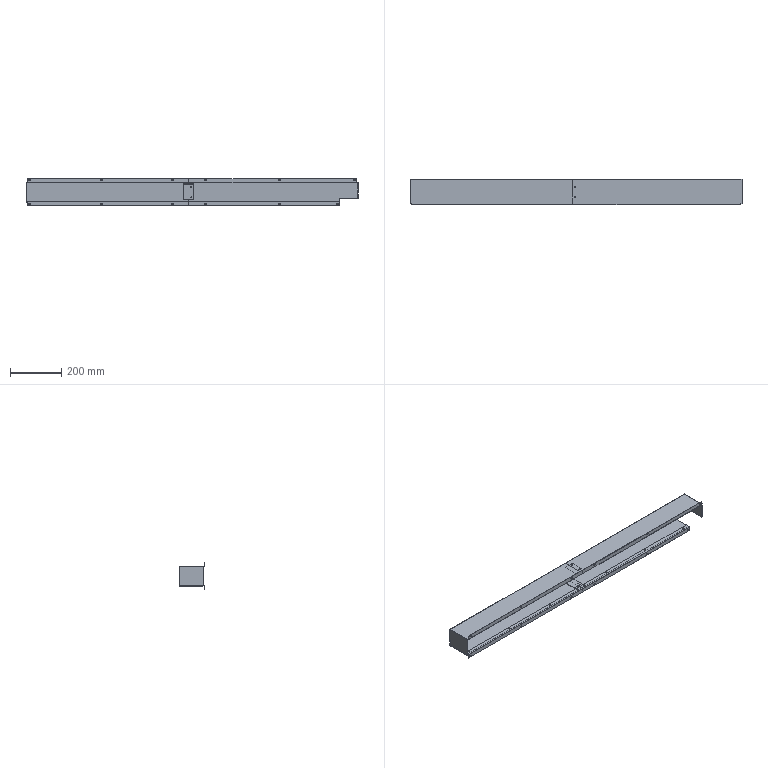Part | STEP file | 0243_226_Cover | 9 solids | 178 faces | box 1302 x 99 x 105 mm | volume 796517 mm3 | plane 98 | cylinder 80 | commonest cylinder face diameters 5 x52 3.3 x28